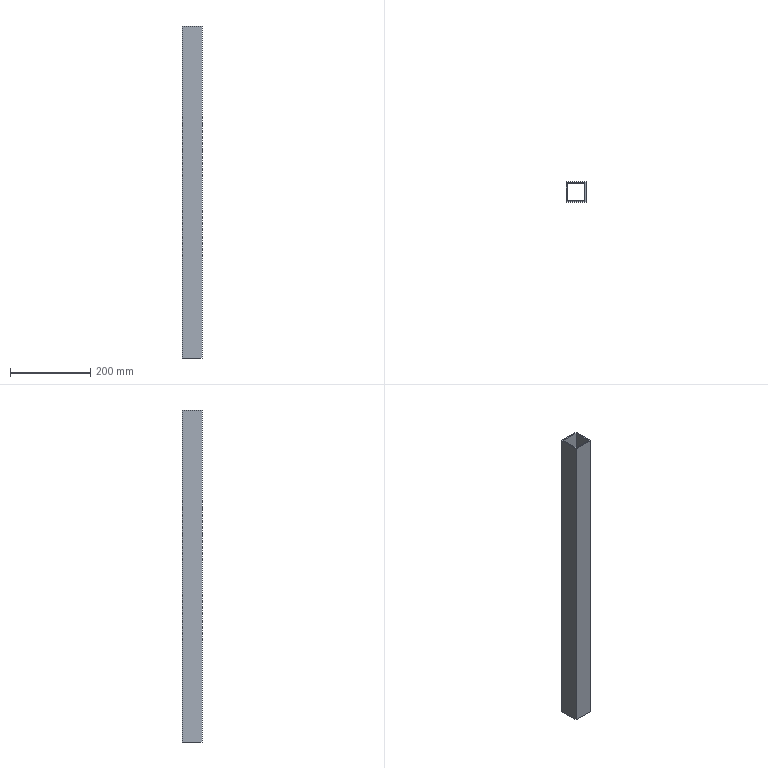Part | STEP file | BCC3 H19_3 | 1 solid | 10 faces | box 50 x 50 x 830 mm | volume 468120 mm3 | plane 10
STEP:
#1=CARTESIAN_POINT('',(0.,0.,0.));
#2=DIRECTION('',(0.,0.,1.));
#3=DIRECTION('',(1.,0.,0.));
#4=AXIS2_PLACEMENT_3D('',#1,#2,#3);
#5=CARTESIAN_POINT('',(-25.,25.,415.));
#6=VERTEX_POINT('',#5);
#7=CARTESIAN_POINT('',(-25.,-25.,415.));
#8=VERTEX_POINT('',#7);
#9=CARTESIAN_POINT('',(-25.,25.,415.));
#10=DIRECTION('',(0.,-1.,0.));
#11=VECTOR('',#10,1.);
#12=LINE('',#9,#11);
#13=CARTESIAN_POINT('',(0.,0.,415.));
#14=DIRECTION('',(0.,0.,1.));
#15=DIRECTION('',(1.,0.,0.));
#16=AXIS2_PLACEMENT_3D('',#13,#14,#15);
#17=PLANE('',#16);
#18=CARTESIAN_POINT('',(-25.,25.));
#19=DIRECTION('',(0.,-1.));
#20=VECTOR('',#19,1.);
#21=LINE('',#18,#20);
#22=(GEOMETRIC_REPRESENTATION_CONTEXT(2)PARAMETRIC_REPRESENTATION_CONTEXT()REPRESENTATION_CONTEXT('',''));
#23=DEFINITIONAL_REPRESENTATION('',(#21),#22);
#24=PCURVE('',#17,#23);
#25=CARTESIAN_POINT('',(-25.,25.,415.));
#26=DIRECTION('',(1.,0.,0.));
#27=DIRECTION('',(0.,1.,0.));
#28=AXIS2_PLACEMENT_3D('',#25,#26,#27);
#29=PLANE('',#28);
#30=CARTESIAN_POINT('',(0.,0.));
#31=DIRECTION('',(-1.,0.));
#32=VECTOR('',#31,1.);
#33=LINE('',#30,#32);
#34=(GEOMETRIC_REPRESENTATION_CONTEXT(2)PARAMETRIC_REPRESENTATION_CONTEXT()REPRESENTATION_CONTEXT('',''));
#35=DEFINITIONAL_REPRESENTATION('',(#33),#34);
#36=PCURVE('',#29,#35);
#37=SURFACE_CURVE('',#12,(#24,#36),.PCURVE_S1.);
#38=EDGE_CURVE('',#6,#8,#37,.T.);
#39=ORIENTED_EDGE('',*,*,#38,.T.);
#40=CARTESIAN_POINT('',(25.,-25.,415.));
#41=VERTEX_POINT('',#40);
#42=CARTESIAN_POINT('',(-25.,-25.,415.));
#43=DIRECTION('',(1.,0.,0.));
#44=VECTOR('',#43,1.);
#45=LINE('',#42,#44);
#46=CARTESIAN_POINT('',(-25.,-25.));
#47=DIRECTION('',(1.,0.));
#48=VECTOR('',#47,1.);
#49=LINE('',#46,#48);
#50=(GEOMETRIC_REPRESENTATION_CONTEXT(2)PARAMETRIC_REPRESENTATION_CONTEXT()REPRESENTATION_CONTEXT('',''));
#51=DEFINITIONAL_REPRESENTATION('',(#49),#50);
#52=PCURVE('',#17,#51);
#53=CARTESIAN_POINT('',(-25.,-25.,415.));
#54=DIRECTION('',(0.,1.,0.));
#55=DIRECTION('',(0.,0.,1.));
#56=AXIS2_PLACEMENT_3D('',#53,#54,#55);
#57=PLANE('',#56);
#58=CARTESIAN_POINT('',(0.,0.));
#59=DIRECTION('',(0.,1.));
#60=VECTOR('',#59,1.);
#61=LINE('',#58,#60);
#62=(GEOMETRIC_REPRESENTATION_CONTEXT(2)PARAMETRIC_REPRESENTATION_CONTEXT()REPRESENTATION_CONTEXT('',''));
#63=DEFINITIONAL_REPRESENTATION('',(#61),#62);
#64=PCURVE('',#57,#63);
#65=SURFACE_CURVE('',#45,(#52,#64),.PCURVE_S1.);
#66=EDGE_CURVE('',#8,#41,#65,.T.);
#67=ORIENTED_EDGE('',*,*,#66,.T.);
#68=CARTESIAN_POINT('',(25.,25.,415.));
#69=VERTEX_POINT('',#68);
#70=CARTESIAN_POINT('',(25.,25.,415.));
#71=DIRECTION('',(0.,1.,0.));
#72=VECTOR('',#71,1.);
#73=LINE('',#70,#72);
#74=CARTESIAN_POINT('',(25.,25.));
#75=DIRECTION('',(0.,1.));
#76=VECTOR('',#75,1.);
#77=LINE('',#74,#76);
#78=(GEOMETRIC_REPRESENTATION_CONTEXT(2)PARAMETRIC_REPRESENTATION_CONTEXT()REPRESENTATION_CONTEXT('',''));
#79=DEFINITIONAL_REPRESENTATION('',(#77),#78);
#80=PCURVE('',#17,#79);
#81=CARTESIAN_POINT('',(25.,25.,415.));
#82=DIRECTION('',(-1.,0.,0.));
#83=DIRECTION('',(0.,-1.,0.));
#84=AXIS2_PLACEMENT_3D('',#81,#82,#83);
#85=PLANE('',#84);
#86=CARTESIAN_POINT('',(0.,0.));
#87=DIRECTION('',(-1.,0.));
#88=VECTOR('',#87,1.);
#89=LINE('',#86,#88);
#90=(GEOMETRIC_REPRESENTATION_CONTEXT(2)PARAMETRIC_REPRESENTATION_CONTEXT()REPRESENTATION_CONTEXT('',''));
#91=DEFINITIONAL_REPRESENTATION('',(#89),#90);
#92=PCURVE('',#85,#91);
#93=SURFACE_CURVE('',#73,(#80,#92),.PCURVE_S1.);
#94=EDGE_CURVE('',#41,#69,#93,.T.);
#95=ORIENTED_EDGE('',*,*,#94,.T.);
#96=CARTESIAN_POINT('',(-25.,25.,415.));
#97=DIRECTION('',(-1.,0.,0.));
#98=VECTOR('',#97,1.);
#99=LINE('',#96,#98);
#100=CARTESIAN_POINT('',(-25.,25.));
#101=DIRECTION('',(-1.,0.));
#102=VECTOR('',#101,1.);
#103=LINE('',#100,#102);
#104=(GEOMETRIC_REPRESENTATION_CONTEXT(2)PARAMETRIC_REPRESENTATION_CONTEXT()REPRESENTATION_CONTEXT('',''));
#105=DEFINITIONAL_REPRESENTATION('',(#103),#104);
#106=PCURVE('',#17,#105);
#107=CARTESIAN_POINT('',(-25.,25.,415.));
#108=DIRECTION('',(0.,-1.,0.));
#109=DIRECTION('',(0.,0.,-1.));
#110=AXIS2_PLACEMENT_3D('',#107,#108,#109);
#111=PLANE('',#110);
#112=CARTESIAN_POINT('',(0.,0.));
#113=DIRECTION('',(0.,-1.));
#114=VECTOR('',#113,1.);
#115=LINE('',#112,#114);
#116=(GEOMETRIC_REPRESENTATION_CONTEXT(2)PARAMETRIC_REPRESENTATION_CONTEXT()REPRESENTATION_CONTEXT('',''));
#117=DEFINITIONAL_REPRESENTATION('',(#115),#116);
#118=PCURVE('',#111,#117);
#119=SURFACE_CURVE('',#99,(#106,#118),.PCURVE_S1.);
#120=EDGE_CURVE('',#69,#6,#119,.T.);
#121=ORIENTED_EDGE('',*,*,#120,.T.);
#122=EDGE_LOOP('',(#39,#67,#95,#121));
#123=FACE_BOUND('',#122,.T.);
#124=CARTESIAN_POINT('',(-22.,-22.,415.));
#125=VERTEX_POINT('',#124);
#126=CARTESIAN_POINT('',(22.,-22.,415.));
#127=VERTEX_POINT('',#126);
#128=CARTESIAN_POINT('',(-22.,-22.,415.));
#129=DIRECTION('',(1.,0.,0.));
#130=VECTOR('',#129,1.);
#131=LINE('',#128,#130);
#132=CARTESIAN_POINT('',(-22.,-22.));
#133=DIRECTION('',(1.,0.));
#134=VECTOR('',#133,1.);
#135=LINE('',#132,#134);
#136=(GEOMETRIC_REPRESENTATION_CONTEXT(2)PARAMETRIC_REPRESENTATION_CONTEXT()REPRESENTATION_CONTEXT('',''));
#137=DEFINITIONAL_REPRESENTATION('',(#135),#136);
#138=PCURVE('',#17,#137);
#139=CARTESIAN_POINT('',(-22.,-22.,415.));
#140=DIRECTION('',(0.,1.,0.));
#141=DIRECTION('',(-1.,0.,0.));
#142=AXIS2_PLACEMENT_3D('',#139,#140,#141);
#143=PLANE('',#142);
#144=CARTESIAN_POINT('',(0.,0.));
#145=DIRECTION('',(-1.,0.));
#146=VECTOR('',#145,1.);
#147=LINE('',#144,#146);
#148=(GEOMETRIC_REPRESENTATION_CONTEXT(2)PARAMETRIC_REPRESENTATION_CONTEXT()REPRESENTATION_CONTEXT('',''));
#149=DEFINITIONAL_REPRESENTATION('',(#147),#148);
#150=PCURVE('',#143,#149);
#151=SURFACE_CURVE('',#131,(#138,#150),.PCURVE_S1.);
#152=EDGE_CURVE('',#125,#127,#151,.T.);
#153=ORIENTED_EDGE('',*,*,#152,.F.);
#154=CARTESIAN_POINT('',(-22.,22.,415.));
#155=VERTEX_POINT('',#154);
#156=CARTESIAN_POINT('',(-22.,22.,415.));
#157=DIRECTION('',(0.,-1.,0.));
#158=VECTOR('',#157,1.);
#159=LINE('',#156,#158);
#160=CARTESIAN_POINT('',(-22.,22.));
#161=DIRECTION('',(0.,-1.));
#162=VECTOR('',#161,1.);
#163=LINE('',#160,#162);
#164=(GEOMETRIC_REPRESENTATION_CONTEXT(2)PARAMETRIC_REPRESENTATION_CONTEXT()REPRESENTATION_CONTEXT('',''));
#165=DEFINITIONAL_REPRESENTATION('',(#163),#164);
#166=PCURVE('',#17,#165);
#167=CARTESIAN_POINT('',(-22.,22.,415.));
#168=DIRECTION('',(1.,0.,0.));
#169=DIRECTION('',(0.,1.,0.));
#170=AXIS2_PLACEMENT_3D('',#167,#168,#169);
#171=PLANE('',#170);
#172=CARTESIAN_POINT('',(0.,0.));
#173=DIRECTION('',(-1.,0.));
#174=VECTOR('',#173,1.);
#175=LINE('',#172,#174);
#176=(GEOMETRIC_REPRESENTATION_CONTEXT(2)PARAMETRIC_REPRESENTATION_CONTEXT()REPRESENTATION_CONTEXT('',''));
#177=DEFINITIONAL_REPRESENTATION('',(#175),#176);
#178=PCURVE('',#171,#177);
#179=SURFACE_CURVE('',#159,(#166,#178),.PCURVE_S1.);
#180=EDGE_CURVE('',#155,#125,#179,.T.);
#181=ORIENTED_EDGE('',*,*,#180,.F.);
#182=CARTESIAN_POINT('',(22.,22.,415.));
#183=VERTEX_POINT('',#182);
#184=CARTESIAN_POINT('',(-22.,22.,415.));
#185=DIRECTION('',(-1.,0.,0.));
#186=VECTOR('',#185,1.);
#187=LINE('',#184,#186);
#188=CARTESIAN_POINT('',(-22.,22.));
#189=DIRECTION('',(-1.,0.));
#190=VECTOR('',#189,1.);
#191=LINE('',#188,#190);
#192=(GEOMETRIC_REPRESENTATION_CONTEXT(2)PARAMETRIC_REPRESENTATION_CONTEXT()REPRESENTATION_CONTEXT('',''));
#193=DEFINITIONAL_REPRESENTATION('',(#191),#192);
#194=PCURVE('',#17,#193);
#195=CARTESIAN_POINT('',(-22.,22.,415.));
#196=DIRECTION('',(0.,-1.,0.));
#197=DIRECTION('',(0.,0.,-1.));
#198=AXIS2_PLACEMENT_3D('',#195,#196,#197);
#199=PLANE('',#198);
#200=CARTESIAN_POINT('',(0.,0.));
#201=DIRECTION('',(0.,-1.));
#202=VECTOR('',#201,1.);
#203=LINE('',#200,#202);
#204=(GEOMETRIC_REPRESENTATION_CONTEXT(2)PARAMETRIC_REPRESENTATION_CONTEXT()REPRESENTATION_CONTEXT('',''));
#205=DEFINITIONAL_REPRESENTATION('',(#203),#204);
#206=PCURVE('',#199,#205);
#207=SURFACE_CURVE('',#187,(#194,#206),.PCURVE_S1.);
#208=EDGE_CURVE('',#183,#155,#207,.T.);
#209=ORIENTED_EDGE('',*,*,#208,.F.);
#210=CARTESIAN_POINT('',(22.,22.,415.));
#211=DIRECTION('',(0.,1.,0.));
#212=VECTOR('',#211,1.);
#213=LINE('',#210,#212);
#214=CARTESIAN_POINT('',(22.,22.));
#215=DIRECTION('',(0.,1.));
#216=VECTOR('',#215,1.);
#217=LINE('',#214,#216);
#218=(GEOMETRIC_REPRESENTATION_CONTEXT(2)PARAMETRIC_REPRESENTATION_CONTEXT()REPRESENTATION_CONTEXT('',''));
#219=DEFINITIONAL_REPRESENTATION('',(#217),#218);
#220=PCURVE('',#17,#219);
#221=CARTESIAN_POINT('',(22.,22.,415.));
#222=DIRECTION('',(-1.,0.,0.));
#223=DIRECTION('',(0.,-1.,0.));
#224=AXIS2_PLACEMENT_3D('',#221,#222,#223);
#225=PLANE('',#224);
#226=CARTESIAN_POINT('',(0.,0.));
#227=DIRECTION('',(-1.,0.));
#228=VECTOR('',#227,1.);
#229=LINE('',#226,#228);
#230=(GEOMETRIC_REPRESENTATION_CONTEXT(2)PARAMETRIC_REPRESENTATION_CONTEXT()REPRESENTATION_CONTEXT('',''));
#231=DEFINITIONAL_REPRESENTATION('',(#229),#230);
#232=PCURVE('',#225,#231);
#233=SURFACE_CURVE('',#213,(#220,#232),.PCURVE_S1.);
#234=EDGE_CURVE('',#127,#183,#233,.T.);
#235=ORIENTED_EDGE('',*,*,#234,.F.);
#236=EDGE_LOOP('',(#153,#181,#209,#235));
#237=FACE_BOUND('',#236,.T.);
#238=ADVANCED_FACE('',(#123,#237),#17,.T.);
#239=CARTESIAN_POINT('',(-25.,25.,-415.));
#240=VERTEX_POINT('',#239);
#241=CARTESIAN_POINT('',(-25.,-25.,-415.));
#242=VERTEX_POINT('',#241);
#243=CARTESIAN_POINT('',(-25.,25.,-415.));
#244=DIRECTION('',(0.,-1.,0.));
#245=VECTOR('',#244,1.);
#246=LINE('',#243,#245);
#247=CARTESIAN_POINT('',(0.,0.,-415.));
#248=DIRECTION('',(0.,0.,1.));
#249=DIRECTION('',(1.,0.,0.));
#250=AXIS2_PLACEMENT_3D('',#247,#248,#249);
#251=PLANE('',#250);
#252=CARTESIAN_POINT('',(-25.,25.));
#253=DIRECTION('',(0.,-1.));
#254=VECTOR('',#253,1.);
#255=LINE('',#252,#254);
#256=(GEOMETRIC_REPRESENTATION_CONTEXT(2)PARAMETRIC_REPRESENTATION_CONTEXT()REPRESENTATION_CONTEXT('',''));
#257=DEFINITIONAL_REPRESENTATION('',(#255),#256);
#258=PCURVE('',#251,#257);
#259=CARTESIAN_POINT('',(0.,-830.));
#260=DIRECTION('',(-1.,0.));
#261=VECTOR('',#260,1.);
#262=LINE('',#259,#261);
#263=(GEOMETRIC_REPRESENTATION_CONTEXT(2)PARAMETRIC_REPRESENTATION_CONTEXT()REPRESENTATION_CONTEXT('',''));
#264=DEFINITIONAL_REPRESENTATION('',(#262),#263);
#265=PCURVE('',#29,#264);
#266=SURFACE_CURVE('',#246,(#258,#265),.PCURVE_S1.);
#267=EDGE_CURVE('',#240,#242,#266,.T.);
#268=ORIENTED_EDGE('',*,*,#267,.F.);
#269=CARTESIAN_POINT('',(25.,25.,-415.));
#270=VERTEX_POINT('',#269);
#271=CARTESIAN_POINT('',(-25.,25.,-415.));
#272=DIRECTION('',(-1.,0.,0.));
#273=VECTOR('',#272,1.);
#274=LINE('',#271,#273);
#275=CARTESIAN_POINT('',(-25.,25.));
#276=DIRECTION('',(-1.,0.));
#277=VECTOR('',#276,1.);
#278=LINE('',#275,#277);
#279=(GEOMETRIC_REPRESENTATION_CONTEXT(2)PARAMETRIC_REPRESENTATION_CONTEXT()REPRESENTATION_CONTEXT('',''));
#280=DEFINITIONAL_REPRESENTATION('',(#278),#279);
#281=PCURVE('',#251,#280);
#282=CARTESIAN_POINT('',(830.,0.));
#283=DIRECTION('',(0.,-1.));
#284=VECTOR('',#283,1.);
#285=LINE('',#282,#284);
#286=(GEOMETRIC_REPRESENTATION_CONTEXT(2)PARAMETRIC_REPRESENTATION_CONTEXT()REPRESENTATION_CONTEXT('',''));
#287=DEFINITIONAL_REPRESENTATION('',(#285),#286);
#288=PCURVE('',#111,#287);
#289=SURFACE_CURVE('',#274,(#281,#288),.PCURVE_S1.);
#290=EDGE_CURVE('',#270,#240,#289,.T.);
#291=ORIENTED_EDGE('',*,*,#290,.F.);
#292=CARTESIAN_POINT('',(25.,-25.,-415.));
#293=VERTEX_POINT('',#292);
#294=CARTESIAN_POINT('',(25.,25.,-415.));
#295=DIRECTION('',(0.,1.,0.));
#296=VECTOR('',#295,1.);
#297=LINE('',#294,#296);
#298=CARTESIAN_POINT('',(25.,25.));
#299=DIRECTION('',(0.,1.));
#300=VECTOR('',#299,1.);
#301=LINE('',#298,#300);
#302=(GEOMETRIC_REPRESENTATION_CONTEXT(2)PARAMETRIC_REPRESENTATION_CONTEXT()REPRESENTATION_CONTEXT('',''));
#303=DEFINITIONAL_REPRESENTATION('',(#301),#302);
#304=PCURVE('',#251,#303);
#305=CARTESIAN_POINT('',(0.,-830.));
#306=DIRECTION('',(-1.,0.));
#307=VECTOR('',#306,1.);
#308=LINE('',#305,#307);
#309=(GEOMETRIC_REPRESENTATION_CONTEXT(2)PARAMETRIC_REPRESENTATION_CONTEXT()REPRESENTATION_CONTEXT('',''));
#310=DEFINITIONAL_REPRESENTATION('',(#308),#309);
#311=PCURVE('',#85,#310);
#312=SURFACE_CURVE('',#297,(#304,#311),.PCURVE_S1.);
#313=EDGE_CURVE('',#293,#270,#312,.T.);
#314=ORIENTED_EDGE('',*,*,#313,.F.);
#315=CARTESIAN_POINT('',(-25.,-25.,-415.));
#316=DIRECTION('',(1.,0.,0.));
#317=VECTOR('',#316,1.);
#318=LINE('',#315,#317);
#319=CARTESIAN_POINT('',(-25.,-25.));
#320=DIRECTION('',(1.,0.));
#321=VECTOR('',#320,1.);
#322=LINE('',#319,#321);
#323=(GEOMETRIC_REPRESENTATION_CONTEXT(2)PARAMETRIC_REPRESENTATION_CONTEXT()REPRESENTATION_CONTEXT('',''));
#324=DEFINITIONAL_REPRESENTATION('',(#322),#323);
#325=PCURVE('',#251,#324);
#326=CARTESIAN_POINT('',(-830.,0.));
#327=DIRECTION('',(0.,1.));
#328=VECTOR('',#327,1.);
#329=LINE('',#326,#328);
#330=(GEOMETRIC_REPRESENTATION_CONTEXT(2)PARAMETRIC_REPRESENTATION_CONTEXT()REPRESENTATION_CONTEXT('',''));
#331=DEFINITIONAL_REPRESENTATION('',(#329),#330);
#332=PCURVE('',#57,#331);
#333=SURFACE_CURVE('',#318,(#325,#332),.PCURVE_S1.);
#334=EDGE_CURVE('',#242,#293,#333,.T.);
#335=ORIENTED_EDGE('',*,*,#334,.F.);
#336=EDGE_LOOP('',(#268,#291,#314,#335));
#337=FACE_BOUND('',#336,.T.);
#338=CARTESIAN_POINT('',(-22.,22.,-415.));
#339=VERTEX_POINT('',#338);
#340=CARTESIAN_POINT('',(-22.,-22.,-415.));
#341=VERTEX_POINT('',#340);
#342=CARTESIAN_POINT('',(-22.,22.,-415.));
#343=DIRECTION('',(0.,-1.,0.));
#344=VECTOR('',#343,1.);
#345=LINE('',#342,#344);
#346=CARTESIAN_POINT('',(-22.,22.));
#347=DIRECTION('',(0.,-1.));
#348=VECTOR('',#347,1.);
#349=LINE('',#346,#348);
#350=(GEOMETRIC_REPRESENTATION_CONTEXT(2)PARAMETRIC_REPRESENTATION_CONTEXT()REPRESENTATION_CONTEXT('',''));
#351=DEFINITIONAL_REPRESENTATION('',(#349),#350);
#352=PCURVE('',#251,#351);
#353=CARTESIAN_POINT('',(0.,-830.));
#354=DIRECTION('',(-1.,0.));
#355=VECTOR('',#354,1.);
#356=LINE('',#353,#355);
#357=(GEOMETRIC_REPRESENTATION_CONTEXT(2)PARAMETRIC_REPRESENTATION_CONTEXT()REPRESENTATION_CONTEXT('',''));
#358=DEFINITIONAL_REPRESENTATION('',(#356),#357);
#359=PCURVE('',#171,#358);
#360=SURFACE_CURVE('',#345,(#352,#359),.PCURVE_S1.);
#361=EDGE_CURVE('',#339,#341,#360,.T.);
#362=ORIENTED_EDGE('',*,*,#361,.T.);
#363=CARTESIAN_POINT('',(22.,-22.,-415.));
#364=VERTEX_POINT('',#363);
#365=CARTESIAN_POINT('',(-22.,-22.,-415.));
#366=DIRECTION('',(1.,0.,0.));
#367=VECTOR('',#366,1.);
#368=LINE('',#365,#367);
#369=CARTESIAN_POINT('',(-22.,-22.));
#370=DIRECTION('',(1.,0.));
#371=VECTOR('',#370,1.);
#372=LINE('',#369,#371);
#373=(GEOMETRIC_REPRESENTATION_CONTEXT(2)PARAMETRIC_REPRESENTATION_CONTEXT()REPRESENTATION_CONTEXT('',''));
#374=DEFINITIONAL_REPRESENTATION('',(#372),#373);
#375=PCURVE('',#251,#374);
#376=CARTESIAN_POINT('',(0.,-830.));
#377=DIRECTION('',(-1.,0.));
#378=VECTOR('',#377,1.);
#379=LINE('',#376,#378);
#380=(GEOMETRIC_REPRESENTATION_CONTEXT(2)PARAMETRIC_REPRESENTATION_CONTEXT()REPRESENTATION_CONTEXT('',''));
#381=DEFINITIONAL_REPRESENTATION('',(#379),#380);
#382=PCURVE('',#143,#381);
#383=SURFACE_CURVE('',#368,(#375,#382),.PCURVE_S1.);
#384=EDGE_CURVE('',#341,#364,#383,.T.);
#385=ORIENTED_EDGE('',*,*,#384,.T.);
#386=CARTESIAN_POINT('',(22.,22.,-415.));
#387=VERTEX_POINT('',#386);
#388=CARTESIAN_POINT('',(22.,22.,-415.));
#389=DIRECTION('',(0.,1.,0.));
#390=VECTOR('',#389,1.);
#391=LINE('',#388,#390);
#392=CARTESIAN_POINT('',(22.,22.));
#393=DIRECTION('',(0.,1.));
#394=VECTOR('',#393,1.);
#395=LINE('',#392,#394);
#396=(GEOMETRIC_REPRESENTATION_CONTEXT(2)PARAMETRIC_REPRESENTATION_CONTEXT()REPRESENTATION_CONTEXT('',''));
#397=DEFINITIONAL_REPRESENTATION('',(#395),#396);
#398=PCURVE('',#251,#397);
#399=CARTESIAN_POINT('',(0.,-830.));
#400=DIRECTION('',(-1.,0.));
#401=VECTOR('',#400,1.);
#402=LINE('',#399,#401);
#403=(GEOMETRIC_REPRESENTATION_CONTEXT(2)PARAMETRIC_REPRESENTATION_CONTEXT()REPRESENTATION_CONTEXT('',''));
#404=DEFINITIONAL_REPRESENTATION('',(#402),#403);
#405=PCURVE('',#225,#404);
#406=SURFACE_CURVE('',#391,(#398,#405),.PCURVE_S1.);
#407=EDGE_CURVE('',#364,#387,#406,.T.);
#408=ORIENTED_EDGE('',*,*,#407,.T.);
#409=CARTESIAN_POINT('',(-22.,22.,-415.));
#410=DIRECTION('',(-1.,0.,0.));
#411=VECTOR('',#410,1.);
#412=LINE('',#409,#411);
#413=CARTESIAN_POINT('',(-22.,22.));
#414=DIRECTION('',(-1.,0.));
#415=VECTOR('',#414,1.);
#416=LINE('',#413,#415);
#417=(GEOMETRIC_REPRESENTATION_CONTEXT(2)PARAMETRIC_REPRESENTATION_CONTEXT()REPRESENTATION_CONTEXT('',''));
#418=DEFINITIONAL_REPRESENTATION('',(#416),#417);
#419=PCURVE('',#251,#418);
#420=CARTESIAN_POINT('',(830.,0.));
#421=DIRECTION('',(0.,-1.));
#422=VECTOR('',#421,1.);
#423=LINE('',#420,#422);
#424=(GEOMETRIC_REPRESENTATION_CONTEXT(2)PARAMETRIC_REPRESENTATION_CONTEXT()REPRESENTATION_CONTEXT('',''));
#425=DEFINITIONAL_REPRESENTATION('',(#423),#424);
#426=PCURVE('',#199,#425);
#427=SURFACE_CURVE('',#412,(#419,#426),.PCURVE_S1.);
#428=EDGE_CURVE('',#387,#339,#427,.T.);
#429=ORIENTED_EDGE('',*,*,#428,.T.);
#430=EDGE_LOOP('',(#362,#385,#408,#429));
#431=FACE_BOUND('',#430,.T.);
#432=ADVANCED_FACE('',(#337,#431),#251,.F.);
#433=ORIENTED_EDGE('',*,*,#267,.T.);
#434=CARTESIAN_POINT('',(-25.,-25.,415.));
#435=DIRECTION('',(0.,0.,-1.));
#436=VECTOR('',#435,1.);
#437=LINE('',#434,#436);
#438=CARTESIAN_POINT('',(-50.,0.));
#439=DIRECTION('',(0.,-1.));
#440=VECTOR('',#439,1.);
#441=LINE('',#438,#440);
#442=(GEOMETRIC_REPRESENTATION_CONTEXT(2)PARAMETRIC_REPRESENTATION_CONTEXT()REPRESENTATION_CONTEXT('',''));
#443=DEFINITIONAL_REPRESENTATION('',(#441),#442);
#444=PCURVE('',#29,#443);
#445=CARTESIAN_POINT('',(0.,0.));
#446=DIRECTION('',(-1.,0.));
#447=VECTOR('',#446,1.);
#448=LINE('',#445,#447);
#449=(GEOMETRIC_REPRESENTATION_CONTEXT(2)PARAMETRIC_REPRESENTATION_CONTEXT()REPRESENTATION_CONTEXT('',''));
#450=DEFINITIONAL_REPRESENTATION('',(#448),#449);
#451=PCURVE('',#57,#450);
#452=SURFACE_CURVE('',#437,(#444,#451),.PCURVE_S1.);
#453=EDGE_CURVE('',#8,#242,#452,.T.);
#454=ORIENTED_EDGE('',*,*,#453,.F.);
#455=ORIENTED_EDGE('',*,*,#38,.F.);
#456=CARTESIAN_POINT('',(-25.,25.,415.));
#457=DIRECTION('',(0.,0.,-1.));
#458=VECTOR('',#457,1.);
#459=LINE('',#456,#458);
#460=CARTESIAN_POINT('',(0.,0.));
#461=DIRECTION('',(0.,-1.));
#462=VECTOR('',#461,1.);
#463=LINE('',#460,#462);
#464=(GEOMETRIC_REPRESENTATION_CONTEXT(2)PARAMETRIC_REPRESENTATION_CONTEXT()REPRESENTATION_CONTEXT('',''));
#465=DEFINITIONAL_REPRESENTATION('',(#463),#464);
#466=PCURVE('',#29,#465);
#467=CARTESIAN_POINT('',(0.,0.));
#468=DIRECTION('',(1.,0.));
#469=VECTOR('',#468,1.);
#470=LINE('',#467,#469);
#471=(GEOMETRIC_REPRESENTATION_CONTEXT(2)PARAMETRIC_REPRESENTATION_CONTEXT()REPRESENTATION_CONTEXT('',''));
#472=DEFINITIONAL_REPRESENTATION('',(#470),#471);
#473=PCURVE('',#111,#472);
#474=SURFACE_CURVE('',#459,(#466,#473),.PCURVE_S1.);
#475=EDGE_CURVE('',#6,#240,#474,.T.);
#476=ORIENTED_EDGE('',*,*,#475,.T.);
#477=EDGE_LOOP('',(#433,#454,#455,#476));
#478=FACE_BOUND('',#477,.T.);
#479=ADVANCED_FACE('',(#478),#29,.F.);
#480=ORIENTED_EDGE('',*,*,#334,.T.);
#481=CARTESIAN_POINT('',(25.,-25.,415.));
#482=DIRECTION('',(0.,0.,-1.));
#483=VECTOR('',#482,1.);
#484=LINE('',#481,#483);
#485=CARTESIAN_POINT('',(0.,50.));
#486=DIRECTION('',(-1.,0.));
#487=VECTOR('',#486,1.);
#488=LINE('',#485,#487);
#489=(GEOMETRIC_REPRESENTATION_CONTEXT(2)PARAMETRIC_REPRESENTATION_CONTEXT()REPRESENTATION_CONTEXT('',''));
#490=DEFINITIONAL_REPRESENTATION('',(#488),#489);
#491=PCURVE('',#57,#490);
#492=CARTESIAN_POINT('',(50.,0.));
#493=DIRECTION('',(0.,-1.));
#494=VECTOR('',#493,1.);
#495=LINE('',#492,#494);
#496=(GEOMETRIC_REPRESENTATION_CONTEXT(2)PARAMETRIC_REPRESENTATION_CONTEXT()REPRESENTATION_CONTEXT('',''));
#497=DEFINITIONAL_REPRESENTATION('',(#495),#496);
#498=PCURVE('',#85,#497);
#499=SURFACE_CURVE('',#484,(#491,#498),.PCURVE_S1.);
#500=EDGE_CURVE('',#41,#293,#499,.T.);
#501=ORIENTED_EDGE('',*,*,#500,.F.);
#502=ORIENTED_EDGE('',*,*,#66,.F.);
#503=ORIENTED_EDGE('',*,*,#453,.T.);
#504=EDGE_LOOP('',(#480,#501,#502,#503));
#505=FACE_BOUND('',#504,.T.);
#506=ADVANCED_FACE('',(#505),#57,.F.);
#507=ORIENTED_EDGE('',*,*,#313,.T.);
#508=CARTESIAN_POINT('',(25.,25.,415.));
#509=DIRECTION('',(0.,0.,-1.));
#510=VECTOR('',#509,1.);
#511=LINE('',#508,#510);
#512=CARTESIAN_POINT('',(0.,0.));
#513=DIRECTION('',(0.,-1.));
#514=VECTOR('',#513,1.);
#515=LINE('',#512,#514);
#516=(GEOMETRIC_REPRESENTATION_CONTEXT(2)PARAMETRIC_REPRESENTATION_CONTEXT()REPRESENTATION_CONTEXT('',''));
#517=DEFINITIONAL_REPRESENTATION('',(#515),#516);
#518=PCURVE('',#85,#517);
#519=CARTESIAN_POINT('',(0.,50.));
#520=DIRECTION('',(1.,0.));
#521=VECTOR('',#520,1.);
#522=LINE('',#519,#521);
#523=(GEOMETRIC_REPRESENTATION_CONTEXT(2)PARAMETRIC_REPRESENTATION_CONTEXT()REPRESENTATION_CONTEXT('',''));
#524=DEFINITIONAL_REPRESENTATION('',(#522),#523);
#525=PCURVE('',#111,#524);
#526=SURFACE_CURVE('',#511,(#518,#525),.PCURVE_S1.);
#527=EDGE_CURVE('',#69,#270,#526,.T.);
#528=ORIENTED_EDGE('',*,*,#527,.F.);
#529=ORIENTED_EDGE('',*,*,#94,.F.);
#530=ORIENTED_EDGE('',*,*,#500,.T.);
#531=EDGE_LOOP('',(#507,#528,#529,#530));
#532=FACE_BOUND('',#531,.T.);
#533=ADVANCED_FACE('',(#532),#85,.F.);
#534=ORIENTED_EDGE('',*,*,#290,.T.);
#535=ORIENTED_EDGE('',*,*,#475,.F.);
#536=ORIENTED_EDGE('',*,*,#120,.F.);
#537=ORIENTED_EDGE('',*,*,#527,.T.);
#538=EDGE_LOOP('',(#534,#535,#536,#537));
#539=FACE_BOUND('',#538,.T.);
#540=ADVANCED_FACE('',(#539),#111,.F.);
#541=ORIENTED_EDGE('',*,*,#361,.F.);
#542=CARTESIAN_POINT('',(-22.,22.,415.));
#543=DIRECTION('',(0.,0.,-1.));
#544=VECTOR('',#543,1.);
#545=LINE('',#542,#544);
#546=CARTESIAN_POINT('',(0.,0.));
#547=DIRECTION('',(0.,-1.));
#548=VECTOR('',#547,1.);
#549=LINE('',#546,#548);
#550=(GEOMETRIC_REPRESENTATION_CONTEXT(2)PARAMETRIC_REPRESENTATION_CONTEXT()REPRESENTATION_CONTEXT('',''));
#551=DEFINITIONAL_REPRESENTATION('',(#549),#550);
#552=PCURVE('',#171,#551);
#553=CARTESIAN_POINT('',(0.,0.));
#554=DIRECTION('',(1.,0.));
#555=VECTOR('',#554,1.);
#556=LINE('',#553,#555);
#557=(GEOMETRIC_REPRESENTATION_CONTEXT(2)PARAMETRIC_REPRESENTATION_CONTEXT()REPRESENTATION_CONTEXT('',''));
#558=DEFINITIONAL_REPRESENTATION('',(#556),#557);
#559=PCURVE('',#199,#558);
#560=SURFACE_CURVE('',#545,(#552,#559),.PCURVE_S1.);
#561=EDGE_CURVE('',#155,#339,#560,.T.);
#562=ORIENTED_EDGE('',*,*,#561,.F.);
#563=ORIENTED_EDGE('',*,*,#180,.T.);
#564=CARTESIAN_POINT('',(-22.,-22.,415.));
#565=DIRECTION('',(0.,0.,-1.));
#566=VECTOR('',#565,1.);
#567=LINE('',#564,#566);
#568=CARTESIAN_POINT('',(-44.,0.));
#569=DIRECTION('',(0.,-1.));
#570=VECTOR('',#569,1.);
#571=LINE('',#568,#570);
#572=(GEOMETRIC_REPRESENTATION_CONTEXT(2)PARAMETRIC_REPRESENTATION_CONTEXT()REPRESENTATION_CONTEXT('',''));
#573=DEFINITIONAL_REPRESENTATION('',(#571),#572);
#574=PCURVE('',#171,#573);
#575=CARTESIAN_POINT('',(0.,0.));
#576=DIRECTION('',(0.,-1.));
#577=VECTOR('',#576,1.);
#578=LINE('',#575,#577);
#579=(GEOMETRIC_REPRESENTATION_CONTEXT(2)PARAMETRIC_REPRESENTATION_CONTEXT()REPRESENTATION_CONTEXT('',''));
#580=DEFINITIONAL_REPRESENTATION('',(#578),#579);
#581=PCURVE('',#143,#580);
#582=SURFACE_CURVE('',#567,(#574,#581),.PCURVE_S1.);
#583=EDGE_CURVE('',#125,#341,#582,.T.);
#584=ORIENTED_EDGE('',*,*,#583,.T.);
#585=EDGE_LOOP('',(#541,#562,#563,#584));
#586=FACE_BOUND('',#585,.T.);
#587=ADVANCED_FACE('',(#586),#171,.T.);
#588=ORIENTED_EDGE('',*,*,#384,.F.);
#589=ORIENTED_EDGE('',*,*,#583,.F.);
#590=ORIENTED_EDGE('',*,*,#152,.T.);
#591=CARTESIAN_POINT('',(22.,-22.,415.));
#592=DIRECTION('',(0.,0.,-1.));
#593=VECTOR('',#592,1.);
#594=LINE('',#591,#593);
#595=CARTESIAN_POINT('',(-44.,0.));
#596=DIRECTION('',(0.,-1.));
#597=VECTOR('',#596,1.);
#598=LINE('',#595,#597);
#599=(GEOMETRIC_REPRESENTATION_CONTEXT(2)PARAMETRIC_REPRESENTATION_CONTEXT()REPRESENTATION_CONTEXT('',''));
#600=DEFINITIONAL_REPRESENTATION('',(#598),#599);
#601=PCURVE('',#143,#600);
#602=CARTESIAN_POINT('',(44.,0.));
#603=DIRECTION('',(0.,-1.));
#604=VECTOR('',#603,1.);
#605=LINE('',#602,#604);
#606=(GEOMETRIC_REPRESENTATION_CONTEXT(2)PARAMETRIC_REPRESENTATION_CONTEXT()REPRESENTATION_CONTEXT('',''));
#607=DEFINITIONAL_REPRESENTATION('',(#605),#606);
#608=PCURVE('',#225,#607);
#609=SURFACE_CURVE('',#594,(#601,#608),.PCURVE_S1.);
#610=EDGE_CURVE('',#127,#364,#609,.T.);
#611=ORIENTED_EDGE('',*,*,#610,.T.);
#612=EDGE_LOOP('',(#588,#589,#590,#611));
#613=FACE_BOUND('',#612,.T.);
#614=ADVANCED_FACE('',(#613),#143,.T.);
#615=ORIENTED_EDGE('',*,*,#407,.F.);
#616=ORIENTED_EDGE('',*,*,#610,.F.);
#617=ORIENTED_EDGE('',*,*,#234,.T.);
#618=CARTESIAN_POINT('',(22.,22.,415.));
#619=DIRECTION('',(0.,0.,-1.));
#620=VECTOR('',#619,1.);
#621=LINE('',#618,#620);
#622=CARTESIAN_POINT('',(0.,0.));
#623=DIRECTION('',(0.,-1.));
#624=VECTOR('',#623,1.);
#625=LINE('',#622,#624);
#626=(GEOMETRIC_REPRESENTATION_CONTEXT(2)PARAMETRIC_REPRESENTATION_CONTEXT()REPRESENTATION_CONTEXT('',''));
#627=DEFINITIONAL_REPRESENTATION('',(#625),#626);
#628=PCURVE('',#225,#627);
#629=CARTESIAN_POINT('',(0.,44.));
#630=DIRECTION('',(1.,0.));
#631=VECTOR('',#630,1.);
#632=LINE('',#629,#631);
#633=(GEOMETRIC_REPRESENTATION_CONTEXT(2)PARAMETRIC_REPRESENTATION_CONTEXT()REPRESENTATION_CONTEXT('',''));
#634=DEFINITIONAL_REPRESENTATION('',(#632),#633);
#635=PCURVE('',#199,#634);
#636=SURFACE_CURVE('',#621,(#628,#635),.PCURVE_S1.);
#637=EDGE_CURVE('',#183,#387,#636,.T.);
#638=ORIENTED_EDGE('',*,*,#637,.T.);
#639=EDGE_LOOP('',(#615,#616,#617,#638));
#640=FACE_BOUND('',#639,.T.);
#641=ADVANCED_FACE('',(#640),#225,.T.);
#642=ORIENTED_EDGE('',*,*,#428,.F.);
#643=ORIENTED_EDGE('',*,*,#637,.F.);
#644=ORIENTED_EDGE('',*,*,#208,.T.);
#645=ORIENTED_EDGE('',*,*,#561,.T.);
#646=EDGE_LOOP('',(#642,#643,#644,#645));
#647=FACE_BOUND('',#646,.T.);
#648=ADVANCED_FACE('',(#647),#199,.T.);
#649=CLOSED_SHELL('',(#238,#432,#479,#506,#533,#540,#587,#614,#641,#648));
#650=MANIFOLD_SOLID_BREP('',#649);
#651=(LENGTH_UNIT()NAMED_UNIT(*)SI_UNIT(.MILLI.,.METRE.));
#652=UNCERTAINTY_MEASURE_WITH_UNIT(LENGTH_MEASURE(0.0000001),#651,'','');
#653=(NAMED_UNIT(*)PLANE_ANGLE_UNIT()SI_UNIT($,.RADIAN.));
#654=(NAMED_UNIT(*)SI_UNIT($,.STERADIAN.)SOLID_ANGLE_UNIT());
#655=(GEOMETRIC_REPRESENTATION_CONTEXT(3)GLOBAL_UNCERTAINTY_ASSIGNED_CONTEXT((#652))GLOBAL_UNIT_ASSIGNED_CONTEXT((#651,#653,#654))REPRESENTATION_CONTEXT('',''));
#656=ADVANCED_BREP_SHAPE_REPRESENTATION('',(#4,#650),#655);